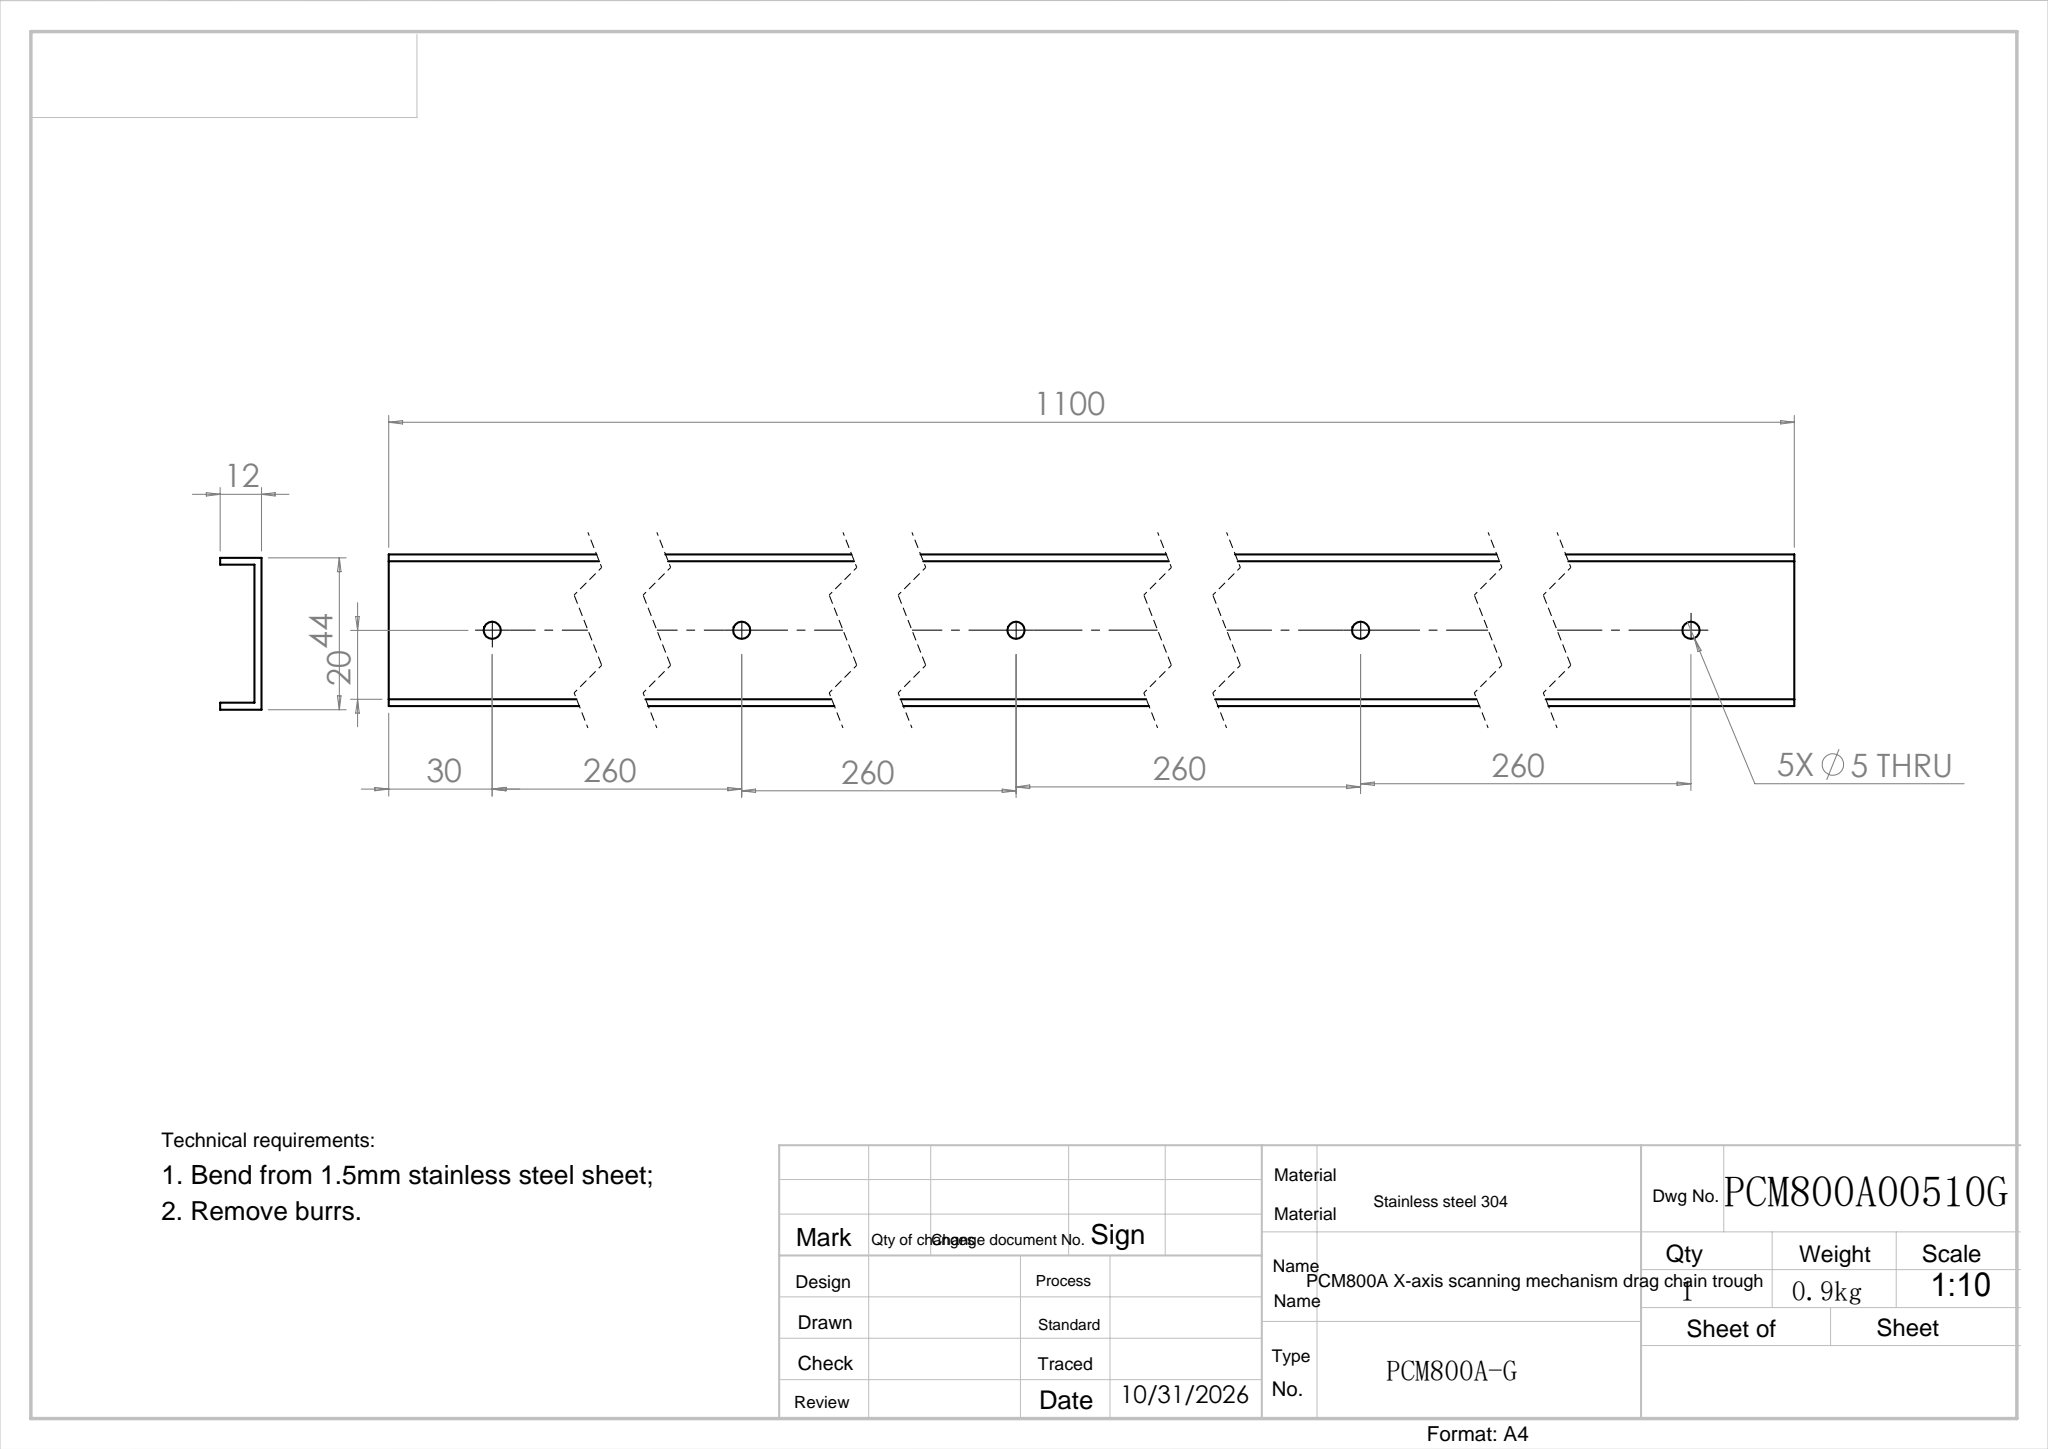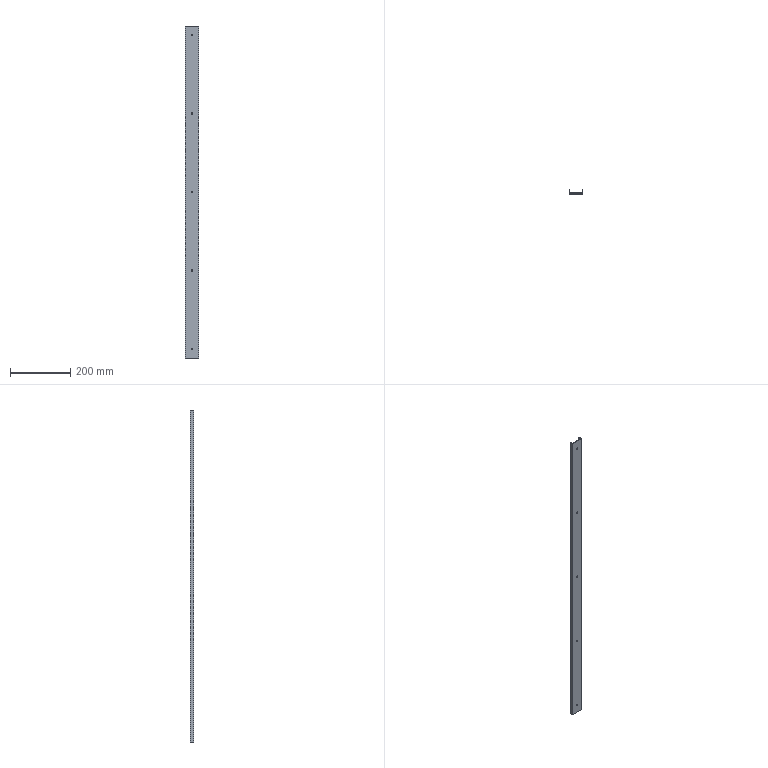Part | SolidWorks | features Extrusion 1, ICE 1, LPattern 1 | 1 solid | 20 faces | box 44 x 12 x 1100 mm | volume 140604 mm3 | cylinder 10 | plane 10 | commonest cylinder face diameters 5 x10
STEP:
#1=CARTESIAN_POINT('',(20.,-12.,1067.5));
#2=VERTEX_POINT('',#1);
#3=CARTESIAN_POINT('',(20.,-12.,1072.5));
#4=VERTEX_POINT('',#3);
#5=CARTESIAN_POINT('',(20.,-12.,1070.));
#6=DIRECTION('',(0.,1.,0.));
#7=DIRECTION('',(0.,0.,1.));
#8=AXIS2_PLACEMENT_3D('',#5,#6,#7);
#9=CIRCLE('',#8,2.5);
#10=EDGE_CURVE('',#2,#4,#9,.T.);
#11=ORIENTED_EDGE('',*,*,#10,.F.);
#12=CARTESIAN_POINT('',(20.,-10.,1067.5));
#13=VERTEX_POINT('',#12);
#14=CARTESIAN_POINT('',(20.,-12.,1067.5));
#15=DIRECTION('',(0.,1.,0.));
#16=VECTOR('',#15,1000.);
#17=LINE('',#14,#16);
#18=EDGE_CURVE('',#2,#13,#17,.T.);
#19=ORIENTED_EDGE('',*,*,#18,.T.);
#20=CARTESIAN_POINT('',(20.,-10.,1072.5));
#21=VERTEX_POINT('',#20);
#22=CARTESIAN_POINT('',(20.,-10.,1070.));
#23=DIRECTION('',(0.,1.,0.));
#24=DIRECTION('',(0.,0.,1.));
#25=AXIS2_PLACEMENT_3D('',#22,#23,#24);
#26=CIRCLE('',#25,2.5);
#27=EDGE_CURVE('',#13,#21,#26,.T.);
#28=ORIENTED_EDGE('',*,*,#27,.T.);
#29=CARTESIAN_POINT('',(20.,-12.,1072.5));
#30=DIRECTION('',(0.,1.,0.));
#31=VECTOR('',#30,1000.);
#32=LINE('',#29,#31);
#33=EDGE_CURVE('',#4,#21,#32,.T.);
#34=ORIENTED_EDGE('',*,*,#33,.F.);
#35=EDGE_LOOP('',(#11,#19,#28,#34));
#36=FACE_OUTER_BOUND('',#35,.T.);
#37=CARTESIAN_POINT('',(20.,-12.,1070.));
#38=DIRECTION('',(0.,1.,0.));
#39=DIRECTION('',(0.,0.,1.));
#40=AXIS2_PLACEMENT_3D('',#37,#38,#39);
#41=CYLINDRICAL_SURFACE('',#40,2.5);
#42=ADVANCED_FACE('',(#36),#41,.F.);
#43=CARTESIAN_POINT('',(20.,-12.,807.5));
#44=VERTEX_POINT('',#43);
#45=CARTESIAN_POINT('',(20.,-12.,812.5));
#46=VERTEX_POINT('',#45);
#47=CARTESIAN_POINT('',(20.,-12.,810.));
#48=DIRECTION('',(0.,1.,0.));
#49=DIRECTION('',(0.,0.,1.));
#50=AXIS2_PLACEMENT_3D('',#47,#48,#49);
#51=CIRCLE('',#50,2.5);
#52=EDGE_CURVE('',#44,#46,#51,.T.);
#53=ORIENTED_EDGE('',*,*,#52,.F.);
#54=CARTESIAN_POINT('',(20.,-10.,807.5));
#55=VERTEX_POINT('',#54);
#56=CARTESIAN_POINT('',(20.,-12.,807.5));
#57=DIRECTION('',(0.,1.,0.));
#58=VECTOR('',#57,1000.);
#59=LINE('',#56,#58);
#60=EDGE_CURVE('',#44,#55,#59,.T.);
#61=ORIENTED_EDGE('',*,*,#60,.T.);
#62=CARTESIAN_POINT('',(20.,-10.,812.5));
#63=VERTEX_POINT('',#62);
#64=CARTESIAN_POINT('',(20.,-10.,810.));
#65=DIRECTION('',(0.,1.,0.));
#66=DIRECTION('',(0.,0.,1.));
#67=AXIS2_PLACEMENT_3D('',#64,#65,#66);
#68=CIRCLE('',#67,2.5);
#69=EDGE_CURVE('',#55,#63,#68,.T.);
#70=ORIENTED_EDGE('',*,*,#69,.T.);
#71=CARTESIAN_POINT('',(20.,-12.,812.5));
#72=DIRECTION('',(0.,1.,0.));
#73=VECTOR('',#72,1000.);
#74=LINE('',#71,#73);
#75=EDGE_CURVE('',#46,#63,#74,.T.);
#76=ORIENTED_EDGE('',*,*,#75,.F.);
#77=EDGE_LOOP('',(#53,#61,#70,#76));
#78=FACE_OUTER_BOUND('',#77,.T.);
#79=CARTESIAN_POINT('',(20.,-12.,810.));
#80=DIRECTION('',(0.,1.,0.));
#81=DIRECTION('',(0.,0.,1.));
#82=AXIS2_PLACEMENT_3D('',#79,#80,#81);
#83=CYLINDRICAL_SURFACE('',#82,2.5);
#84=ADVANCED_FACE('',(#78),#83,.F.);
#85=CARTESIAN_POINT('',(20.,-12.,547.5));
#86=VERTEX_POINT('',#85);
#87=CARTESIAN_POINT('',(20.,-12.,552.5));
#88=VERTEX_POINT('',#87);
#89=CARTESIAN_POINT('',(20.,-12.,550.));
#90=DIRECTION('',(0.,1.,0.));
#91=DIRECTION('',(0.,0.,1.));
#92=AXIS2_PLACEMENT_3D('',#89,#90,#91);
#93=CIRCLE('',#92,2.5);
#94=EDGE_CURVE('',#86,#88,#93,.T.);
#95=ORIENTED_EDGE('',*,*,#94,.F.);
#96=CARTESIAN_POINT('',(20.,-10.,547.5));
#97=VERTEX_POINT('',#96);
#98=CARTESIAN_POINT('',(20.,-12.,547.5));
#99=DIRECTION('',(0.,1.,0.));
#100=VECTOR('',#99,1000.);
#101=LINE('',#98,#100);
#102=EDGE_CURVE('',#86,#97,#101,.T.);
#103=ORIENTED_EDGE('',*,*,#102,.T.);
#104=CARTESIAN_POINT('',(20.,-10.,552.5));
#105=VERTEX_POINT('',#104);
#106=CARTESIAN_POINT('',(20.,-10.,550.));
#107=DIRECTION('',(0.,1.,0.));
#108=DIRECTION('',(0.,0.,1.));
#109=AXIS2_PLACEMENT_3D('',#106,#107,#108);
#110=CIRCLE('',#109,2.5);
#111=EDGE_CURVE('',#97,#105,#110,.T.);
#112=ORIENTED_EDGE('',*,*,#111,.T.);
#113=CARTESIAN_POINT('',(20.,-12.,552.5));
#114=DIRECTION('',(0.,1.,0.));
#115=VECTOR('',#114,1000.);
#116=LINE('',#113,#115);
#117=EDGE_CURVE('',#88,#105,#116,.T.);
#118=ORIENTED_EDGE('',*,*,#117,.F.);
#119=EDGE_LOOP('',(#95,#103,#112,#118));
#120=FACE_OUTER_BOUND('',#119,.T.);
#121=CARTESIAN_POINT('',(20.,-12.,550.));
#122=DIRECTION('',(0.,1.,0.));
#123=DIRECTION('',(0.,0.,1.));
#124=AXIS2_PLACEMENT_3D('',#121,#122,#123);
#125=CYLINDRICAL_SURFACE('',#124,2.5);
#126=ADVANCED_FACE('',(#120),#125,.F.);
#127=CARTESIAN_POINT('',(20.,-12.,287.5));
#128=VERTEX_POINT('',#127);
#129=CARTESIAN_POINT('',(20.,-12.,292.5));
#130=VERTEX_POINT('',#129);
#131=CARTESIAN_POINT('',(20.,-12.,290.));
#132=DIRECTION('',(0.,1.,0.));
#133=DIRECTION('',(0.,0.,1.));
#134=AXIS2_PLACEMENT_3D('',#131,#132,#133);
#135=CIRCLE('',#134,2.5);
#136=EDGE_CURVE('',#128,#130,#135,.T.);
#137=ORIENTED_EDGE('',*,*,#136,.F.);
#138=CARTESIAN_POINT('',(20.,-10.,287.5));
#139=VERTEX_POINT('',#138);
#140=CARTESIAN_POINT('',(20.,-12.,287.5));
#141=DIRECTION('',(0.,1.,0.));
#142=VECTOR('',#141,1000.);
#143=LINE('',#140,#142);
#144=EDGE_CURVE('',#128,#139,#143,.T.);
#145=ORIENTED_EDGE('',*,*,#144,.T.);
#146=CARTESIAN_POINT('',(20.,-10.,292.5));
#147=VERTEX_POINT('',#146);
#148=CARTESIAN_POINT('',(20.,-10.,290.));
#149=DIRECTION('',(0.,1.,0.));
#150=DIRECTION('',(0.,0.,1.));
#151=AXIS2_PLACEMENT_3D('',#148,#149,#150);
#152=CIRCLE('',#151,2.5);
#153=EDGE_CURVE('',#139,#147,#152,.T.);
#154=ORIENTED_EDGE('',*,*,#153,.T.);
#155=CARTESIAN_POINT('',(20.,-12.,292.5));
#156=DIRECTION('',(0.,1.,0.));
#157=VECTOR('',#156,1000.);
#158=LINE('',#155,#157);
#159=EDGE_CURVE('',#130,#147,#158,.T.);
#160=ORIENTED_EDGE('',*,*,#159,.F.);
#161=EDGE_LOOP('',(#137,#145,#154,#160));
#162=FACE_OUTER_BOUND('',#161,.T.);
#163=CARTESIAN_POINT('',(20.,-12.,290.));
#164=DIRECTION('',(0.,1.,0.));
#165=DIRECTION('',(0.,0.,1.));
#166=AXIS2_PLACEMENT_3D('',#163,#164,#165);
#167=CYLINDRICAL_SURFACE('',#166,2.5);
#168=ADVANCED_FACE('',(#162),#167,.F.);
#169=CARTESIAN_POINT('',(20.,-12.,27.5));
#170=VERTEX_POINT('',#169);
#171=CARTESIAN_POINT('',(20.,-12.,32.5));
#172=VERTEX_POINT('',#171);
#173=CARTESIAN_POINT('',(20.,-12.,30.));
#174=DIRECTION('',(0.,1.,0.));
#175=DIRECTION('',(0.,0.,1.));
#176=AXIS2_PLACEMENT_3D('',#173,#174,#175);
#177=CIRCLE('',#176,2.5);
#178=EDGE_CURVE('',#170,#172,#177,.T.);
#179=ORIENTED_EDGE('',*,*,#178,.F.);
#180=CARTESIAN_POINT('',(20.,-10.,27.5));
#181=VERTEX_POINT('',#180);
#182=CARTESIAN_POINT('',(20.,-12.,27.5));
#183=DIRECTION('',(0.,1.,0.));
#184=VECTOR('',#183,1000.);
#185=LINE('',#182,#184);
#186=EDGE_CURVE('',#170,#181,#185,.T.);
#187=ORIENTED_EDGE('',*,*,#186,.T.);
#188=CARTESIAN_POINT('',(20.,-10.,32.5));
#189=VERTEX_POINT('',#188);
#190=CARTESIAN_POINT('',(20.,-10.,30.));
#191=DIRECTION('',(0.,1.,0.));
#192=DIRECTION('',(0.,0.,1.));
#193=AXIS2_PLACEMENT_3D('',#190,#191,#192);
#194=CIRCLE('',#193,2.5);
#195=EDGE_CURVE('',#181,#189,#194,.T.);
#196=ORIENTED_EDGE('',*,*,#195,.T.);
#197=CARTESIAN_POINT('',(20.,-12.,32.5));
#198=DIRECTION('',(0.,1.,0.));
#199=VECTOR('',#198,1000.);
#200=LINE('',#197,#199);
#201=EDGE_CURVE('',#172,#189,#200,.T.);
#202=ORIENTED_EDGE('',*,*,#201,.F.);
#203=EDGE_LOOP('',(#179,#187,#196,#202));
#204=FACE_OUTER_BOUND('',#203,.T.);
#205=CARTESIAN_POINT('',(20.,-12.,30.));
#206=DIRECTION('',(0.,1.,0.));
#207=DIRECTION('',(0.,0.,1.));
#208=AXIS2_PLACEMENT_3D('',#205,#206,#207);
#209=CYLINDRICAL_SURFACE('',#208,2.5);
#210=ADVANCED_FACE('',(#204),#209,.F.);
#211=CARTESIAN_POINT('',(0.,0.,0.));
#212=VERTEX_POINT('',#211);
#213=CARTESIAN_POINT('',(-2.,0.,0.));
#214=VERTEX_POINT('',#213);
#215=CARTESIAN_POINT('',(-2.,0.,0.));
#216=DIRECTION('',(-1.,0.,0.));
#217=VECTOR('',#216,1000.);
#218=LINE('',#215,#217);
#219=EDGE_CURVE('',#212,#214,#218,.T.);
#220=ORIENTED_EDGE('',*,*,#219,.T.);
#221=CARTESIAN_POINT('',(-2.,0.,1100.));
#222=VERTEX_POINT('',#221);
#223=CARTESIAN_POINT('',(-2.,0.,1100.));
#224=DIRECTION('',(0.,0.,-1.));
#225=VECTOR('',#224,1000.);
#226=LINE('',#223,#225);
#227=EDGE_CURVE('',#222,#214,#226,.T.);
#228=ORIENTED_EDGE('',*,*,#227,.F.);
#229=CARTESIAN_POINT('',(0.,0.,1100.));
#230=VERTEX_POINT('',#229);
#231=CARTESIAN_POINT('',(-2.,0.,1100.));
#232=DIRECTION('',(-1.,0.,0.));
#233=VECTOR('',#232,1000.);
#234=LINE('',#231,#233);
#235=EDGE_CURVE('',#230,#222,#234,.T.);
#236=ORIENTED_EDGE('',*,*,#235,.F.);
#237=CARTESIAN_POINT('',(0.,0.,1100.));
#238=DIRECTION('',(0.,0.,-1.));
#239=VECTOR('',#238,1000.);
#240=LINE('',#237,#239);
#241=EDGE_CURVE('',#230,#212,#240,.T.);
#242=ORIENTED_EDGE('',*,*,#241,.T.);
#243=EDGE_LOOP('',(#220,#228,#236,#242));
#244=FACE_OUTER_BOUND('',#243,.T.);
#245=CARTESIAN_POINT('',(-2.,0.,1100.));
#246=DIRECTION('',(0.,-1.,0.));
#247=DIRECTION('',(0.,0.,-1.));
#248=AXIS2_PLACEMENT_3D('',#245,#246,#247);
#249=PLANE('',#248);
#250=ADVANCED_FACE('',(#244),#249,.F.);
#251=CARTESIAN_POINT('',(-2.,-12.,0.));
#252=VERTEX_POINT('',#251);
#253=CARTESIAN_POINT('',(-2.,0.,0.));
#254=DIRECTION('',(0.,-1.,0.));
#255=VECTOR('',#254,1000.);
#256=LINE('',#253,#255);
#257=EDGE_CURVE('',#214,#252,#256,.T.);
#258=ORIENTED_EDGE('',*,*,#257,.T.);
#259=CARTESIAN_POINT('',(-2.,-12.,1100.));
#260=VERTEX_POINT('',#259);
#261=CARTESIAN_POINT('',(-2.,-12.,1100.));
#262=DIRECTION('',(0.,0.,-1.));
#263=VECTOR('',#262,1000.);
#264=LINE('',#261,#263);
#265=EDGE_CURVE('',#260,#252,#264,.T.);
#266=ORIENTED_EDGE('',*,*,#265,.F.);
#267=CARTESIAN_POINT('',(-2.,0.,1100.));
#268=DIRECTION('',(0.,-1.,0.));
#269=VECTOR('',#268,1000.);
#270=LINE('',#267,#269);
#271=EDGE_CURVE('',#222,#260,#270,.T.);
#272=ORIENTED_EDGE('',*,*,#271,.F.);
#273=ORIENTED_EDGE('',*,*,#227,.T.);
#274=EDGE_LOOP('',(#258,#266,#272,#273));
#275=FACE_OUTER_BOUND('',#274,.T.);
#276=CARTESIAN_POINT('',(-2.,0.,1100.));
#277=DIRECTION('',(1.,0.,0.));
#278=DIRECTION('',(0.,0.,-1.));
#279=AXIS2_PLACEMENT_3D('',#276,#277,#278);
#280=PLANE('',#279);
#281=ADVANCED_FACE('',(#275),#280,.F.);
#282=CARTESIAN_POINT('',(20.,-12.,290.));
#283=DIRECTION('',(0.,1.,0.));
#284=DIRECTION('',(0.,0.,1.));
#285=AXIS2_PLACEMENT_3D('',#282,#283,#284);
#286=CIRCLE('',#285,2.5);
#287=EDGE_CURVE('',#130,#128,#286,.T.);
#288=ORIENTED_EDGE('',*,*,#287,.T.);
#289=ORIENTED_EDGE('',*,*,#136,.T.);
#290=EDGE_LOOP('',(#288,#289));
#291=FACE_BOUND('',#290,.T.);
#292=CARTESIAN_POINT('',(20.,-12.,30.));
#293=DIRECTION('',(0.,1.,0.));
#294=DIRECTION('',(0.,0.,1.));
#295=AXIS2_PLACEMENT_3D('',#292,#293,#294);
#296=CIRCLE('',#295,2.5);
#297=EDGE_CURVE('',#172,#170,#296,.T.);
#298=ORIENTED_EDGE('',*,*,#297,.T.);
#299=ORIENTED_EDGE('',*,*,#178,.T.);
#300=EDGE_LOOP('',(#298,#299));
#301=FACE_BOUND('',#300,.T.);
#302=CARTESIAN_POINT('',(42.,-12.,0.));
#303=VERTEX_POINT('',#302);
#304=CARTESIAN_POINT('',(-2.,-12.,0.));
#305=DIRECTION('',(1.,0.,0.));
#306=VECTOR('',#305,1000.);
#307=LINE('',#304,#306);
#308=EDGE_CURVE('',#252,#303,#307,.T.);
#309=ORIENTED_EDGE('',*,*,#308,.T.);
#310=CARTESIAN_POINT('',(42.,-12.,1100.));
#311=VERTEX_POINT('',#310);
#312=CARTESIAN_POINT('',(42.,-12.,1100.));
#313=DIRECTION('',(0.,0.,-1.));
#314=VECTOR('',#313,1000.);
#315=LINE('',#312,#314);
#316=EDGE_CURVE('',#311,#303,#315,.T.);
#317=ORIENTED_EDGE('',*,*,#316,.F.);
#318=CARTESIAN_POINT('',(-2.,-12.,1100.));
#319=DIRECTION('',(1.,0.,0.));
#320=VECTOR('',#319,1000.);
#321=LINE('',#318,#320);
#322=EDGE_CURVE('',#260,#311,#321,.T.);
#323=ORIENTED_EDGE('',*,*,#322,.F.);
#324=ORIENTED_EDGE('',*,*,#265,.T.);
#325=EDGE_LOOP('',(#309,#317,#323,#324));
#326=FACE_OUTER_BOUND('',#325,.T.);
#327=CARTESIAN_POINT('',(20.,-12.,550.));
#328=DIRECTION('',(0.,1.,0.));
#329=DIRECTION('',(0.,0.,1.));
#330=AXIS2_PLACEMENT_3D('',#327,#328,#329);
#331=CIRCLE('',#330,2.5);
#332=EDGE_CURVE('',#88,#86,#331,.T.);
#333=ORIENTED_EDGE('',*,*,#332,.T.);
#334=ORIENTED_EDGE('',*,*,#94,.T.);
#335=EDGE_LOOP('',(#333,#334));
#336=FACE_BOUND('',#335,.T.);
#337=CARTESIAN_POINT('',(20.,-12.,810.));
#338=DIRECTION('',(0.,1.,0.));
#339=DIRECTION('',(0.,0.,1.));
#340=AXIS2_PLACEMENT_3D('',#337,#338,#339);
#341=CIRCLE('',#340,2.5);
#342=EDGE_CURVE('',#46,#44,#341,.T.);
#343=ORIENTED_EDGE('',*,*,#342,.T.);
#344=ORIENTED_EDGE('',*,*,#52,.T.);
#345=EDGE_LOOP('',(#343,#344));
#346=FACE_BOUND('',#345,.T.);
#347=CARTESIAN_POINT('',(20.,-12.,1070.));
#348=DIRECTION('',(0.,1.,0.));
#349=DIRECTION('',(0.,0.,1.));
#350=AXIS2_PLACEMENT_3D('',#347,#348,#349);
#351=CIRCLE('',#350,2.5);
#352=EDGE_CURVE('',#4,#2,#351,.T.);
#353=ORIENTED_EDGE('',*,*,#352,.T.);
#354=ORIENTED_EDGE('',*,*,#10,.T.);
#355=EDGE_LOOP('',(#353,#354));
#356=FACE_BOUND('',#355,.T.);
#357=CARTESIAN_POINT('',(-2.,-12.,1100.));
#358=DIRECTION('',(0.,1.,0.));
#359=DIRECTION('',(0.,0.,1.));
#360=AXIS2_PLACEMENT_3D('',#357,#358,#359);
#361=PLANE('',#360);
#362=ADVANCED_FACE('',(#291,#301,#326,#336,#346,#356),#361,.F.);
#363=CARTESIAN_POINT('',(42.,0.,0.));
#364=VERTEX_POINT('',#363);
#365=CARTESIAN_POINT('',(42.,-12.,0.));
#366=DIRECTION('',(0.,1.,0.));
#367=VECTOR('',#366,1000.);
#368=LINE('',#365,#367);
#369=EDGE_CURVE('',#303,#364,#368,.T.);
#370=ORIENTED_EDGE('',*,*,#369,.T.);
#371=CARTESIAN_POINT('',(42.,0.,1100.));
#372=VERTEX_POINT('',#371);
#373=CARTESIAN_POINT('',(42.,0.,1100.));
#374=DIRECTION('',(0.,0.,-1.));
#375=VECTOR('',#374,1000.);
#376=LINE('',#373,#375);
#377=EDGE_CURVE('',#372,#364,#376,.T.);
#378=ORIENTED_EDGE('',*,*,#377,.F.);
#379=CARTESIAN_POINT('',(42.,-12.,1100.));
#380=DIRECTION('',(0.,1.,0.));
#381=VECTOR('',#380,1000.);
#382=LINE('',#379,#381);
#383=EDGE_CURVE('',#311,#372,#382,.T.);
#384=ORIENTED_EDGE('',*,*,#383,.F.);
#385=ORIENTED_EDGE('',*,*,#316,.T.);
#386=EDGE_LOOP('',(#370,#378,#384,#385));
#387=FACE_OUTER_BOUND('',#386,.T.);
#388=CARTESIAN_POINT('',(42.,-12.,1100.));
#389=DIRECTION('',(-1.,0.,0.));
#390=DIRECTION('',(0.,0.,1.));
#391=AXIS2_PLACEMENT_3D('',#388,#389,#390);
#392=PLANE('',#391);
#393=ADVANCED_FACE('',(#387),#392,.F.);
#394=CARTESIAN_POINT('',(40.,0.,0.));
#395=VERTEX_POINT('',#394);
#396=CARTESIAN_POINT('',(42.,0.,0.));
#397=DIRECTION('',(-1.,0.,0.));
#398=VECTOR('',#397,1000.);
#399=LINE('',#396,#398);
#400=EDGE_CURVE('',#364,#395,#399,.T.);
#401=ORIENTED_EDGE('',*,*,#400,.T.);
#402=CARTESIAN_POINT('',(40.,0.,1100.));
#403=VERTEX_POINT('',#402);
#404=CARTESIAN_POINT('',(40.,0.,1100.));
#405=DIRECTION('',(0.,0.,-1.));
#406=VECTOR('',#405,1000.);
#407=LINE('',#404,#406);
#408=EDGE_CURVE('',#403,#395,#407,.T.);
#409=ORIENTED_EDGE('',*,*,#408,.F.);
#410=CARTESIAN_POINT('',(42.,0.,1100.));
#411=DIRECTION('',(-1.,0.,0.));
#412=VECTOR('',#411,1000.);
#413=LINE('',#410,#412);
#414=EDGE_CURVE('',#372,#403,#413,.T.);
#415=ORIENTED_EDGE('',*,*,#414,.F.);
#416=ORIENTED_EDGE('',*,*,#377,.T.);
#417=EDGE_LOOP('',(#401,#409,#415,#416));
#418=FACE_OUTER_BOUND('',#417,.T.);
#419=CARTESIAN_POINT('',(42.,0.,1100.));
#420=DIRECTION('',(0.,-1.,0.));
#421=DIRECTION('',(1.,0.,0.));
#422=AXIS2_PLACEMENT_3D('',#419,#420,#421);
#423=PLANE('',#422);
#424=ADVANCED_FACE('',(#418),#423,.F.);
#425=CARTESIAN_POINT('',(40.,-10.,0.));
#426=VERTEX_POINT('',#425);
#427=CARTESIAN_POINT('',(40.,0.,0.));
#428=DIRECTION('',(0.,-1.,0.));
#429=VECTOR('',#428,1000.);
#430=LINE('',#427,#429);
#431=EDGE_CURVE('',#395,#426,#430,.T.);
#432=ORIENTED_EDGE('',*,*,#431,.T.);
#433=CARTESIAN_POINT('',(40.,-10.,1100.));
#434=VERTEX_POINT('',#433);
#435=CARTESIAN_POINT('',(40.,-10.,1100.));
#436=DIRECTION('',(0.,0.,-1.));
#437=VECTOR('',#436,1000.);
#438=LINE('',#435,#437);
#439=EDGE_CURVE('',#434,#426,#438,.T.);
#440=ORIENTED_EDGE('',*,*,#439,.F.);
#441=CARTESIAN_POINT('',(40.,0.,1100.));
#442=DIRECTION('',(0.,-1.,0.));
#443=VECTOR('',#442,1000.);
#444=LINE('',#441,#443);
#445=EDGE_CURVE('',#403,#434,#444,.T.);
#446=ORIENTED_EDGE('',*,*,#445,.F.);
#447=ORIENTED_EDGE('',*,*,#408,.T.);
#448=EDGE_LOOP('',(#432,#440,#446,#447));
#449=FACE_OUTER_BOUND('',#448,.T.);
#450=CARTESIAN_POINT('',(40.,0.,1100.));
#451=DIRECTION('',(1.,0.,0.));
#452=DIRECTION('',(0.,0.,-1.));
#453=AXIS2_PLACEMENT_3D('',#450,#451,#452);
#454=PLANE('',#453);
#455=ADVANCED_FACE('',(#449),#454,.F.);
#456=CARTESIAN_POINT('',(20.,-10.,290.));
#457=DIRECTION('',(0.,1.,0.));
#458=DIRECTION('',(0.,0.,1.));
#459=AXIS2_PLACEMENT_3D('',#456,#457,#458);
#460=CIRCLE('',#459,2.5);
#461=EDGE_CURVE('',#147,#139,#460,.T.);
#462=ORIENTED_EDGE('',*,*,#461,.F.);
#463=ORIENTED_EDGE('',*,*,#153,.F.);
#464=EDGE_LOOP('',(#462,#463));
#465=FACE_BOUND('',#464,.T.);
#466=CARTESIAN_POINT('',(20.,-10.,30.));
#467=DIRECTION('',(0.,1.,0.));
#468=DIRECTION('',(0.,0.,1.));
#469=AXIS2_PLACEMENT_3D('',#466,#467,#468);
#470=CIRCLE('',#469,2.5);
#471=EDGE_CURVE('',#189,#181,#470,.T.);
#472=ORIENTED_EDGE('',*,*,#471,.F.);
#473=ORIENTED_EDGE('',*,*,#195,.F.);
#474=EDGE_LOOP('',(#472,#473));
#475=FACE_BOUND('',#474,.T.);
#476=CARTESIAN_POINT('',(0.,-10.,0.));
#477=VERTEX_POINT('',#476);
#478=CARTESIAN_POINT('',(0.,-10.,0.));
#479=DIRECTION('',(-1.,0.,0.));
#480=VECTOR('',#479,1000.);
#481=LINE('',#478,#480);
#482=EDGE_CURVE('',#426,#477,#481,.T.);
#483=ORIENTED_EDGE('',*,*,#482,.T.);
#484=CARTESIAN_POINT('',(0.,-10.,1100.));
#485=VERTEX_POINT('',#484);
#486=CARTESIAN_POINT('',(0.,-10.,1100.));
#487=DIRECTION('',(0.,0.,-1.));
#488=VECTOR('',#487,1000.);
#489=LINE('',#486,#488);
#490=EDGE_CURVE('',#485,#477,#489,.T.);
#491=ORIENTED_EDGE('',*,*,#490,.F.);
#492=CARTESIAN_POINT('',(0.,-10.,1100.));
#493=DIRECTION('',(-1.,0.,0.));
#494=VECTOR('',#493,1000.);
#495=LINE('',#492,#494);
#496=EDGE_CURVE('',#434,#485,#495,.T.);
#497=ORIENTED_EDGE('',*,*,#496,.F.);
#498=ORIENTED_EDGE('',*,*,#439,.T.);
#499=EDGE_LOOP('',(#483,#491,#497,#498));
#500=FACE_OUTER_BOUND('',#499,.T.);
#501=CARTESIAN_POINT('',(20.,-10.,550.));
#502=DIRECTION('',(0.,1.,0.));
#503=DIRECTION('',(0.,0.,1.));
#504=AXIS2_PLACEMENT_3D('',#501,#502,#503);
#505=CIRCLE('',#504,2.5);
#506=EDGE_CURVE('',#105,#97,#505,.T.);
#507=ORIENTED_EDGE('',*,*,#506,.F.);
#508=ORIENTED_EDGE('',*,*,#111,.F.);
#509=EDGE_LOOP('',(#507,#508));
#510=FACE_BOUND('',#509,.T.);
#511=CARTESIAN_POINT('',(20.,-10.,810.));
#512=DIRECTION('',(0.,1.,0.));
#513=DIRECTION('',(0.,0.,1.));
#514=AXIS2_PLACEMENT_3D('',#511,#512,#513);
#515=CIRCLE('',#514,2.5);
#516=EDGE_CURVE('',#63,#55,#515,.T.);
#517=ORIENTED_EDGE('',*,*,#516,.F.);
#518=ORIENTED_EDGE('',*,*,#69,.F.);
#519=EDGE_LOOP('',(#517,#518));
#520=FACE_BOUND('',#519,.T.);
#521=CARTESIAN_POINT('',(20.,-10.,1070.));
#522=DIRECTION('',(0.,1.,0.));
#523=DIRECTION('',(0.,0.,1.));
#524=AXIS2_PLACEMENT_3D('',#521,#522,#523);
#525=CIRCLE('',#524,2.5);
#526=EDGE_CURVE('',#21,#13,#525,.T.);
#527=ORIENTED_EDGE('',*,*,#526,.F.);
#528=ORIENTED_EDGE('',*,*,#27,.F.);
#529=EDGE_LOOP('',(#527,#528));
#530=FACE_BOUND('',#529,.T.);
#531=CARTESIAN_POINT('',(0.,-10.,1100.));
#532=DIRECTION('',(0.,-1.,0.));
#533=DIRECTION('',(0.,0.,-1.));
#534=AXIS2_PLACEMENT_3D('',#531,#532,#533);
#535=PLANE('',#534);
#536=ADVANCED_FACE('',(#465,#475,#500,#510,#520,#530),#535,.F.);
#537=CARTESIAN_POINT('',(0.,0.,0.));
#538=DIRECTION('',(0.,1.,0.));
#539=VECTOR('',#538,1000.);
#540=LINE('',#537,#539);
#541=EDGE_CURVE('',#477,#212,#540,.T.);
#542=ORIENTED_EDGE('',*,*,#541,.T.);
#543=ORIENTED_EDGE('',*,*,#241,.F.);
#544=CARTESIAN_POINT('',(0.,0.,1100.));
#545=DIRECTION('',(0.,1.,0.));
#546=VECTOR('',#545,1000.);
#547=LINE('',#544,#546);
#548=EDGE_CURVE('',#485,#230,#547,.T.);
#549=ORIENTED_EDGE('',*,*,#548,.F.);
#550=ORIENTED_EDGE('',*,*,#490,.T.);
#551=EDGE_LOOP('',(#542,#543,#549,#550));
#552=FACE_OUTER_BOUND('',#551,.T.);
#553=CARTESIAN_POINT('',(0.,0.,1100.));
#554=DIRECTION('',(-1.,0.,0.));
#555=DIRECTION('',(0.,-1.,0.));
#556=AXIS2_PLACEMENT_3D('',#553,#554,#555);
#557=PLANE('',#556);
#558=ADVANCED_FACE('',(#552),#557,.F.);
#559=ORIENTED_EDGE('',*,*,#235,.T.);
#560=ORIENTED_EDGE('',*,*,#271,.T.);
#561=ORIENTED_EDGE('',*,*,#322,.T.);
#562=ORIENTED_EDGE('',*,*,#383,.T.);
#563=ORIENTED_EDGE('',*,*,#414,.T.);
#564=ORIENTED_EDGE('',*,*,#445,.T.);
#565=ORIENTED_EDGE('',*,*,#496,.T.);
#566=ORIENTED_EDGE('',*,*,#548,.T.);
#567=EDGE_LOOP('',(#559,#560,#561,#562,#563,#564,#565,#566));
#568=FACE_OUTER_BOUND('',#567,.T.);
#569=CARTESIAN_POINT('',(0.,0.,1100.));
#570=DIRECTION('',(0.,0.,-1.));
#571=DIRECTION('',(-1.,0.,0.));
#572=AXIS2_PLACEMENT_3D('',#569,#570,#571);
#573=PLANE('',#572);
#574=ADVANCED_FACE('',(#568),#573,.F.);
#575=ORIENTED_EDGE('',*,*,#219,.F.);
#576=ORIENTED_EDGE('',*,*,#541,.F.);
#577=ORIENTED_EDGE('',*,*,#482,.F.);
#578=ORIENTED_EDGE('',*,*,#431,.F.);
#579=ORIENTED_EDGE('',*,*,#400,.F.);
#580=ORIENTED_EDGE('',*,*,#369,.F.);
#581=ORIENTED_EDGE('',*,*,#308,.F.);
#582=ORIENTED_EDGE('',*,*,#257,.F.);
#583=EDGE_LOOP('',(#575,#576,#577,#578,#579,#580,#581,#582));
#584=FACE_OUTER_BOUND('',#583,.T.);
#585=CARTESIAN_POINT('',(0.,0.,0.));
#586=DIRECTION('',(0.,0.,-1.));
#587=DIRECTION('',(-1.,0.,0.));
#588=AXIS2_PLACEMENT_3D('',#585,#586,#587);
#589=PLANE('',#588);
#590=ADVANCED_FACE('',(#584),#589,.T.);
#591=ORIENTED_EDGE('',*,*,#186,.F.);
#592=ORIENTED_EDGE('',*,*,#297,.F.);
#593=ORIENTED_EDGE('',*,*,#201,.T.);
#594=ORIENTED_EDGE('',*,*,#471,.T.);
#595=EDGE_LOOP('',(#591,#592,#593,#594));
#596=FACE_OUTER_BOUND('',#595,.T.);
#597=CARTESIAN_POINT('',(20.,-12.,30.));
#598=DIRECTION('',(0.,1.,0.));
#599=DIRECTION('',(0.,0.,1.));
#600=AXIS2_PLACEMENT_3D('',#597,#598,#599);
#601=CYLINDRICAL_SURFACE('',#600,2.5);
#602=ADVANCED_FACE('',(#596),#601,.F.);
#603=ORIENTED_EDGE('',*,*,#144,.F.);
#604=ORIENTED_EDGE('',*,*,#287,.F.);
#605=ORIENTED_EDGE('',*,*,#159,.T.);
#606=ORIENTED_EDGE('',*,*,#461,.T.);
#607=EDGE_LOOP('',(#603,#604,#605,#606));
#608=FACE_OUTER_BOUND('',#607,.T.);
#609=CARTESIAN_POINT('',(20.,-12.,290.));
#610=DIRECTION('',(0.,1.,0.));
#611=DIRECTION('',(0.,0.,1.));
#612=AXIS2_PLACEMENT_3D('',#609,#610,#611);
#613=CYLINDRICAL_SURFACE('',#612,2.5);
#614=ADVANCED_FACE('',(#608),#613,.F.);
#615=ORIENTED_EDGE('',*,*,#102,.F.);
#616=ORIENTED_EDGE('',*,*,#332,.F.);
#617=ORIENTED_EDGE('',*,*,#117,.T.);
#618=ORIENTED_EDGE('',*,*,#506,.T.);
#619=EDGE_LOOP('',(#615,#616,#617,#618));
#620=FACE_OUTER_BOUND('',#619,.T.);
#621=CARTESIAN_POINT('',(20.,-12.,550.));
#622=DIRECTION('',(0.,1.,0.));
#623=DIRECTION('',(0.,0.,1.));
#624=AXIS2_PLACEMENT_3D('',#621,#622,#623);
#625=CYLINDRICAL_SURFACE('',#624,2.5);
#626=ADVANCED_FACE('',(#620),#625,.F.);
#627=ORIENTED_EDGE('',*,*,#60,.F.);
#628=ORIENTED_EDGE('',*,*,#342,.F.);
#629=ORIENTED_EDGE('',*,*,#75,.T.);
#630=ORIENTED_EDGE('',*,*,#516,.T.);
#631=EDGE_LOOP('',(#627,#628,#629,#630));
#632=FACE_OUTER_BOUND('',#631,.T.);
#633=CARTESIAN_POINT('',(20.,-12.,810.));
#634=DIRECTION('',(0.,1.,0.));
#635=DIRECTION('',(0.,0.,1.));
#636=AXIS2_PLACEMENT_3D('',#633,#634,#635);
#637=CYLINDRICAL_SURFACE('',#636,2.5);
#638=ADVANCED_FACE('',(#632),#637,.F.);
#639=ORIENTED_EDGE('',*,*,#18,.F.);
#640=ORIENTED_EDGE('',*,*,#352,.F.);
#641=ORIENTED_EDGE('',*,*,#33,.T.);
#642=ORIENTED_EDGE('',*,*,#526,.T.);
#643=EDGE_LOOP('',(#639,#640,#641,#642));
#644=FACE_OUTER_BOUND('',#643,.T.);
#645=CARTESIAN_POINT('',(20.,-12.,1070.));
#646=DIRECTION('',(0.,1.,0.));
#647=DIRECTION('',(0.,0.,1.));
#648=AXIS2_PLACEMENT_3D('',#645,#646,#647);
#649=CYLINDRICAL_SURFACE('',#648,2.5);
#650=ADVANCED_FACE('',(#644),#649,.F.);
#651=CLOSED_SHELL('',(#42,#84,#126,#168,#210,#250,#281,#362,#393,#424,#455,#536,#558,#574,#590,#602,#614,#626,#638,#650));
#652=MANIFOLD_SOLID_BREP('',#651);
#653=CARTESIAN_POINT('',(0.,0.,0.));
#654=DIRECTION('',(0.,0.,1.));
#655=DIRECTION('',(1.,0.,0.));
#656=AXIS2_PLACEMENT_3D('',#653,#654,#655);
#657=(LENGTH_UNIT()NAMED_UNIT(*)SI_UNIT(.MILLI.,.METRE.));
#658=UNCERTAINTY_MEASURE_WITH_UNIT(LENGTH_MEASURE(0.00001),#657,'','');
#659=(NAMED_UNIT(*)PLANE_ANGLE_UNIT()SI_UNIT($,.RADIAN.));
#660=(NAMED_UNIT(*)SI_UNIT($,.STERADIAN.)SOLID_ANGLE_UNIT());
#661=(GEOMETRIC_REPRESENTATION_CONTEXT(3)GLOBAL_UNCERTAINTY_ASSIGNED_CONTEXT((#658))GLOBAL_UNIT_ASSIGNED_CONTEXT((#657,#659,#660))REPRESENTATION_CONTEXT('',''));
#662=ADVANCED_BREP_SHAPE_REPRESENTATION('',(#652,#656),#661);